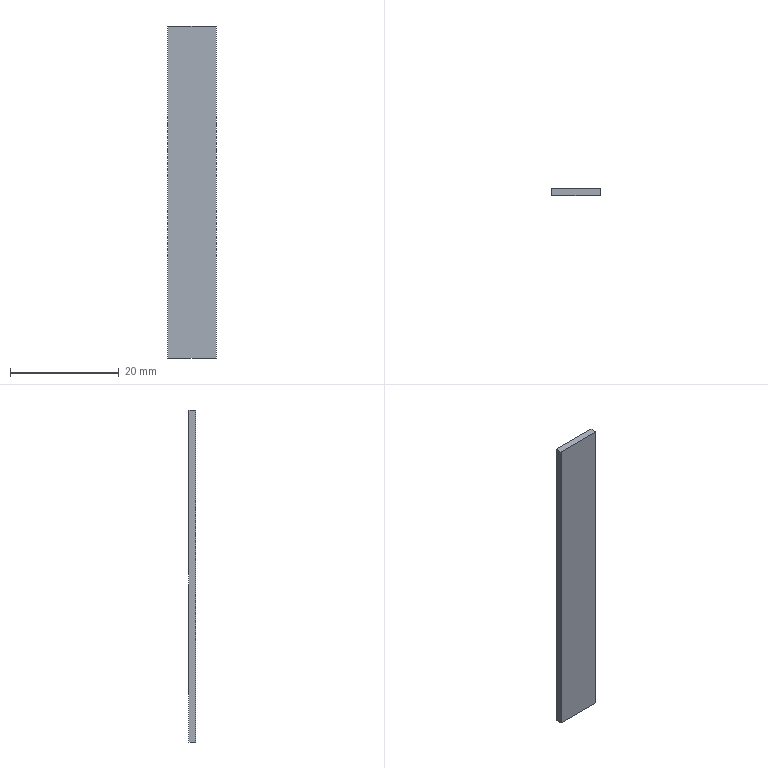Part | SolidWorks | features ICE 3, Extrusion 1 | 1 solid | 121 faces | box 9 x 1.35 x 61 mm | volume 702.043 mm3 | plane 96 | spline 25